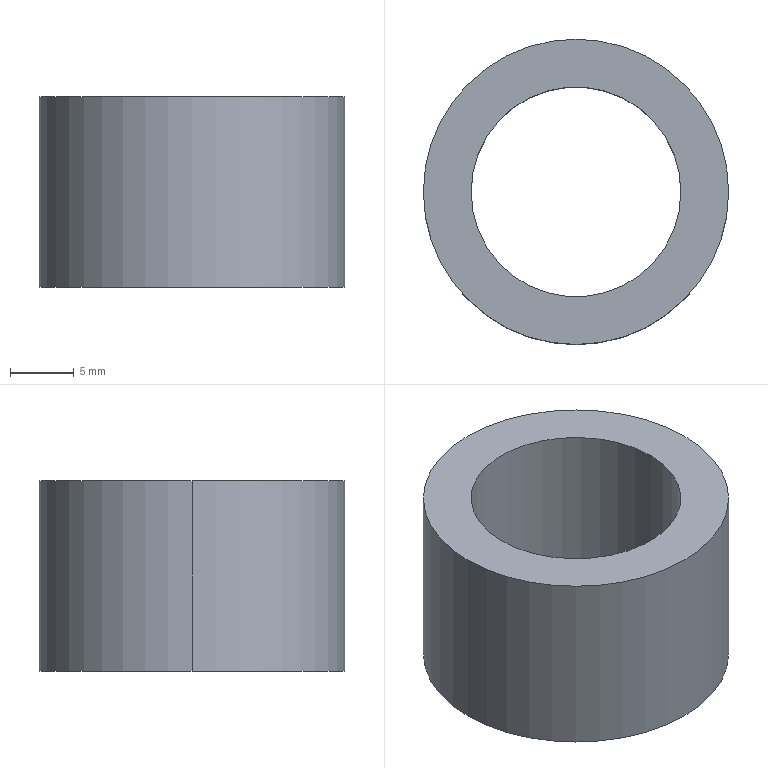Part | SolidWorks | features Extrusion 1 | 1 solid | 6 faces | box 24 x 24 x 15 mm | volume 3578 mm3 | cylinder 4 | plane 2 | commonest cylinder face diameters 16.5 x2 24 x2
STEP:
#1=CARTESIAN_POINT('',(-8.25,0.,15.));
#2=VERTEX_POINT('',#1);
#3=CARTESIAN_POINT('',(8.25,0.,15.));
#4=VERTEX_POINT('',#3);
#5=CARTESIAN_POINT('',(0.,0.,15.));
#6=DIRECTION('',(0.,0.,1.));
#7=DIRECTION('',(1.,0.,0.));
#8=AXIS2_PLACEMENT_3D('',#5,#6,#7);
#9=CIRCLE('',#8,8.25);
#10=EDGE_CURVE('',#2,#4,#9,.T.);
#11=ORIENTED_EDGE('',*,*,#10,.T.);
#12=CARTESIAN_POINT('',(8.25,0.,0.));
#13=VERTEX_POINT('',#12);
#14=CARTESIAN_POINT('',(8.25,0.,15.));
#15=DIRECTION('',(0.,0.,-1.));
#16=VECTOR('',#15,1000.);
#17=LINE('',#14,#16);
#18=EDGE_CURVE('',#4,#13,#17,.T.);
#19=ORIENTED_EDGE('',*,*,#18,.T.);
#20=CARTESIAN_POINT('',(-8.25,0.,0.));
#21=VERTEX_POINT('',#20);
#22=CARTESIAN_POINT('',(0.,0.,0.));
#23=DIRECTION('',(0.,0.,1.));
#24=DIRECTION('',(1.,0.,0.));
#25=AXIS2_PLACEMENT_3D('',#22,#23,#24);
#26=CIRCLE('',#25,8.25);
#27=EDGE_CURVE('',#21,#13,#26,.T.);
#28=ORIENTED_EDGE('',*,*,#27,.F.);
#29=CARTESIAN_POINT('',(-8.25,0.,15.));
#30=DIRECTION('',(0.,0.,-1.));
#31=VECTOR('',#30,1000.);
#32=LINE('',#29,#31);
#33=EDGE_CURVE('',#2,#21,#32,.T.);
#34=ORIENTED_EDGE('',*,*,#33,.F.);
#35=EDGE_LOOP('',(#11,#19,#28,#34));
#36=FACE_OUTER_BOUND('',#35,.T.);
#37=CARTESIAN_POINT('',(0.,0.,15.));
#38=DIRECTION('',(0.,0.,-1.));
#39=DIRECTION('',(-1.,0.,0.));
#40=AXIS2_PLACEMENT_3D('',#37,#38,#39);
#41=CYLINDRICAL_SURFACE('',#40,8.25);
#42=ADVANCED_FACE('',(#36),#41,.F.);
#43=CARTESIAN_POINT('',(12.,0.,15.));
#44=VERTEX_POINT('',#43);
#45=CARTESIAN_POINT('',(-12.,0.,15.));
#46=VERTEX_POINT('',#45);
#47=CARTESIAN_POINT('',(0.,0.,15.));
#48=DIRECTION('',(0.,0.,1.));
#49=DIRECTION('',(1.,0.,0.));
#50=AXIS2_PLACEMENT_3D('',#47,#48,#49);
#51=CIRCLE('',#50,12.);
#52=EDGE_CURVE('',#44,#46,#51,.T.);
#53=ORIENTED_EDGE('',*,*,#52,.F.);
#54=CARTESIAN_POINT('',(12.,0.,0.));
#55=VERTEX_POINT('',#54);
#56=CARTESIAN_POINT('',(12.,0.,15.));
#57=DIRECTION('',(0.,0.,-1.));
#58=VECTOR('',#57,1000.);
#59=LINE('',#56,#58);
#60=EDGE_CURVE('',#44,#55,#59,.T.);
#61=ORIENTED_EDGE('',*,*,#60,.T.);
#62=CARTESIAN_POINT('',(-12.,0.,0.));
#63=VERTEX_POINT('',#62);
#64=CARTESIAN_POINT('',(0.,0.,0.));
#65=DIRECTION('',(0.,0.,1.));
#66=DIRECTION('',(1.,0.,0.));
#67=AXIS2_PLACEMENT_3D('',#64,#65,#66);
#68=CIRCLE('',#67,12.);
#69=EDGE_CURVE('',#55,#63,#68,.T.);
#70=ORIENTED_EDGE('',*,*,#69,.T.);
#71=CARTESIAN_POINT('',(-12.,0.,15.));
#72=DIRECTION('',(0.,0.,-1.));
#73=VECTOR('',#72,1000.);
#74=LINE('',#71,#73);
#75=EDGE_CURVE('',#46,#63,#74,.T.);
#76=ORIENTED_EDGE('',*,*,#75,.F.);
#77=EDGE_LOOP('',(#53,#61,#70,#76));
#78=FACE_OUTER_BOUND('',#77,.T.);
#79=CARTESIAN_POINT('',(0.,0.,15.));
#80=DIRECTION('',(0.,0.,-1.));
#81=DIRECTION('',(-1.,0.,0.));
#82=AXIS2_PLACEMENT_3D('',#79,#80,#81);
#83=CYLINDRICAL_SURFACE('',#82,12.);
#84=ADVANCED_FACE('',(#78),#83,.T.);
#85=CARTESIAN_POINT('',(0.,0.,15.));
#86=DIRECTION('',(0.,0.,1.));
#87=DIRECTION('',(1.,0.,0.));
#88=AXIS2_PLACEMENT_3D('',#85,#86,#87);
#89=CIRCLE('',#88,12.);
#90=EDGE_CURVE('',#46,#44,#89,.T.);
#91=ORIENTED_EDGE('',*,*,#90,.T.);
#92=ORIENTED_EDGE('',*,*,#52,.T.);
#93=EDGE_LOOP('',(#91,#92));
#94=FACE_OUTER_BOUND('',#93,.T.);
#95=ORIENTED_EDGE('',*,*,#10,.F.);
#96=CARTESIAN_POINT('',(0.,0.,15.));
#97=DIRECTION('',(0.,0.,1.));
#98=DIRECTION('',(1.,0.,0.));
#99=AXIS2_PLACEMENT_3D('',#96,#97,#98);
#100=CIRCLE('',#99,8.25);
#101=EDGE_CURVE('',#4,#2,#100,.T.);
#102=ORIENTED_EDGE('',*,*,#101,.F.);
#103=EDGE_LOOP('',(#95,#102));
#104=FACE_BOUND('',#103,.T.);
#105=CARTESIAN_POINT('',(0.,0.,15.));
#106=DIRECTION('',(0.,0.,1.));
#107=DIRECTION('',(1.,0.,0.));
#108=AXIS2_PLACEMENT_3D('',#105,#106,#107);
#109=PLANE('',#108);
#110=ADVANCED_FACE('',(#94,#104),#109,.T.);
#111=CARTESIAN_POINT('',(0.,0.,0.));
#112=DIRECTION('',(0.,0.,1.));
#113=DIRECTION('',(1.,0.,0.));
#114=AXIS2_PLACEMENT_3D('',#111,#112,#113);
#115=CIRCLE('',#114,12.);
#116=EDGE_CURVE('',#63,#55,#115,.T.);
#117=ORIENTED_EDGE('',*,*,#116,.F.);
#118=ORIENTED_EDGE('',*,*,#69,.F.);
#119=EDGE_LOOP('',(#117,#118));
#120=FACE_OUTER_BOUND('',#119,.T.);
#121=ORIENTED_EDGE('',*,*,#27,.T.);
#122=CARTESIAN_POINT('',(0.,0.,0.));
#123=DIRECTION('',(0.,0.,1.));
#124=DIRECTION('',(1.,0.,0.));
#125=AXIS2_PLACEMENT_3D('',#122,#123,#124);
#126=CIRCLE('',#125,8.25);
#127=EDGE_CURVE('',#13,#21,#126,.T.);
#128=ORIENTED_EDGE('',*,*,#127,.T.);
#129=EDGE_LOOP('',(#121,#128));
#130=FACE_BOUND('',#129,.T.);
#131=CARTESIAN_POINT('',(0.,0.,0.));
#132=DIRECTION('',(0.,0.,1.));
#133=DIRECTION('',(1.,0.,0.));
#134=AXIS2_PLACEMENT_3D('',#131,#132,#133);
#135=PLANE('',#134);
#136=ADVANCED_FACE('',(#120,#130),#135,.F.);
#137=ORIENTED_EDGE('',*,*,#60,.F.);
#138=ORIENTED_EDGE('',*,*,#90,.F.);
#139=ORIENTED_EDGE('',*,*,#75,.T.);
#140=ORIENTED_EDGE('',*,*,#116,.T.);
#141=EDGE_LOOP('',(#137,#138,#139,#140));
#142=FACE_OUTER_BOUND('',#141,.T.);
#143=CARTESIAN_POINT('',(0.,0.,15.));
#144=DIRECTION('',(0.,0.,-1.));
#145=DIRECTION('',(-1.,0.,0.));
#146=AXIS2_PLACEMENT_3D('',#143,#144,#145);
#147=CYLINDRICAL_SURFACE('',#146,12.);
#148=ADVANCED_FACE('',(#142),#147,.T.);
#149=ORIENTED_EDGE('',*,*,#18,.F.);
#150=ORIENTED_EDGE('',*,*,#101,.T.);
#151=ORIENTED_EDGE('',*,*,#33,.T.);
#152=ORIENTED_EDGE('',*,*,#127,.F.);
#153=EDGE_LOOP('',(#149,#150,#151,#152));
#154=FACE_OUTER_BOUND('',#153,.T.);
#155=CARTESIAN_POINT('',(0.,0.,15.));
#156=DIRECTION('',(0.,0.,-1.));
#157=DIRECTION('',(-1.,0.,0.));
#158=AXIS2_PLACEMENT_3D('',#155,#156,#157);
#159=CYLINDRICAL_SURFACE('',#158,8.25);
#160=ADVANCED_FACE('',(#154),#159,.F.);
#161=CLOSED_SHELL('',(#42,#84,#110,#136,#148,#160));
#162=MANIFOLD_SOLID_BREP('',#161);
#163=CARTESIAN_POINT('',(0.,0.,0.));
#164=DIRECTION('',(0.,0.,1.));
#165=DIRECTION('',(1.,0.,0.));
#166=AXIS2_PLACEMENT_3D('',#163,#164,#165);
#167=(LENGTH_UNIT()NAMED_UNIT(*)SI_UNIT(.MILLI.,.METRE.));
#168=UNCERTAINTY_MEASURE_WITH_UNIT(LENGTH_MEASURE(0.00001),#167,'','');
#169=(NAMED_UNIT(*)PLANE_ANGLE_UNIT()SI_UNIT($,.RADIAN.));
#170=(NAMED_UNIT(*)SI_UNIT($,.STERADIAN.)SOLID_ANGLE_UNIT());
#171=(GEOMETRIC_REPRESENTATION_CONTEXT(3)GLOBAL_UNCERTAINTY_ASSIGNED_CONTEXT((#168))GLOBAL_UNIT_ASSIGNED_CONTEXT((#167,#169,#170))REPRESENTATION_CONTEXT('',''));
#172=ADVANCED_BREP_SHAPE_REPRESENTATION('',(#162,#166),#171);